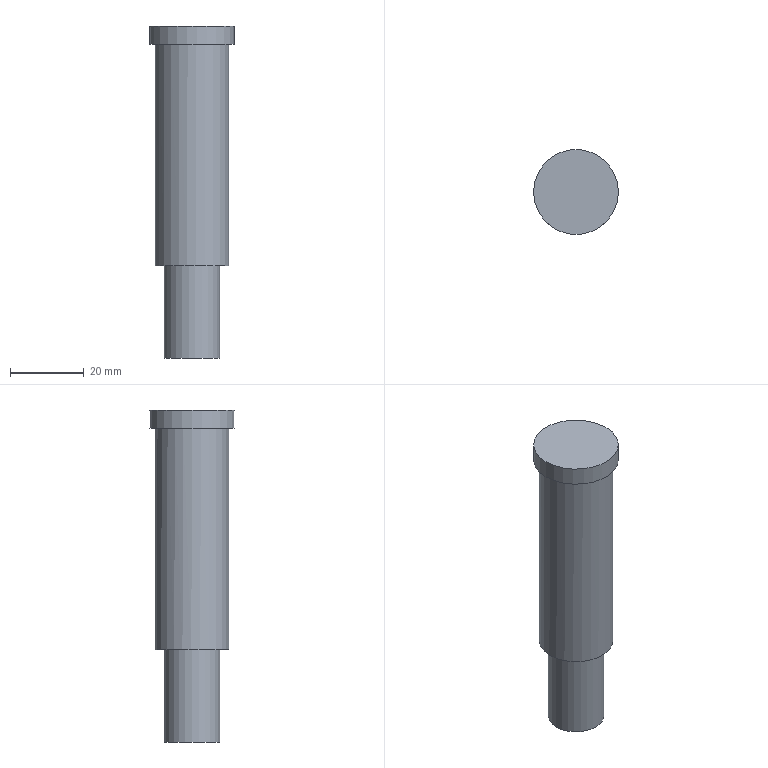Part | NX | features solid 2 | 1 solid | 7 faces | box 23 x 23 x 90 mm | volume 25404 mm3 | plane 4 | cylinder 3 | commonest cylinder face diameters 15.1 x1 20 x1 23 x1
STEP:
#1=CARTESIAN_POINT('',(-704.653,-121.65,86.));
#2=VERTEX_POINT('',#1);
#3=CARTESIAN_POINT('',(-694.993,-124.238,86.));
#4=DIRECTION('',(0.,0.,1.));
#5=DIRECTION('',(-0.9659,0.2588,0.));
#6=AXIS2_PLACEMENT_3D('',#3,#4,#5);
#7=CIRCLE('',#6,10.);
#8=EDGE_CURVE('',#2,#2,#7,.T.);
#9=ORIENTED_EDGE('',*,*,#8,.T.);
#10=EDGE_LOOP('',(#9));
#11=FACE_BOUND('',#10,.T.);
#12=CARTESIAN_POINT('',(-684.993,-124.238,146.));
#13=VERTEX_POINT('',#12);
#14=CARTESIAN_POINT('',(-694.993,-124.238,146.));
#15=DIRECTION('',(0.,0.,1.));
#16=DIRECTION('',(1.,0.,0.));
#17=AXIS2_PLACEMENT_3D('',#14,#15,#16);
#18=CIRCLE('',#17,10.);
#19=EDGE_CURVE('',#13,#13,#18,.T.);
#20=ORIENTED_EDGE('',*,*,#19,.F.);
#21=EDGE_LOOP('',(#20));
#22=FACE_BOUND('',#21,.T.);
#23=CARTESIAN_POINT('',(-694.993,-124.238,141.));
#24=DIRECTION('',(0.,0.,-1.));
#25=DIRECTION('',(0.9659,-0.2588,0.));
#26=AXIS2_PLACEMENT_3D('',#23,#24,#25);
#27=CYLINDRICAL_SURFACE('',#26,10.);
#28=ADVANCED_FACE('',(#11,#22),#27,.T.);
#29=CARTESIAN_POINT('',(-687.443,-124.238,86.));
#30=VERTEX_POINT('',#29);
#31=CARTESIAN_POINT('',(-694.993,-124.238,86.));
#32=DIRECTION('',(0.,0.,1.));
#33=DIRECTION('',(1.,0.,0.));
#34=AXIS2_PLACEMENT_3D('',#31,#32,#33);
#35=CIRCLE('',#34,7.55);
#36=EDGE_CURVE('',#30,#30,#35,.T.);
#37=ORIENTED_EDGE('',*,*,#36,.T.);
#38=EDGE_LOOP('',(#37));
#39=FACE_BOUND('',#38,.T.);
#40=ORIENTED_EDGE('',*,*,#8,.F.);
#41=EDGE_LOOP('',(#40));
#42=FACE_BOUND('',#41,.T.);
#43=CARTESIAN_POINT('',(-694.993,-124.238,86.));
#44=DIRECTION('',(0.,0.,1.));
#45=DIRECTION('',(-0.9659,0.2588,0.));
#46=AXIS2_PLACEMENT_3D('',#43,#44,#45);
#47=PLANE('',#46);
#48=ADVANCED_FACE('',(#39,#42),#47,.F.);
#49=CARTESIAN_POINT('',(-683.493,-124.238,146.));
#50=VERTEX_POINT('',#49);
#51=CARTESIAN_POINT('',(-694.993,-124.238,146.));
#52=DIRECTION('',(0.,0.,1.));
#53=DIRECTION('',(1.,0.,0.));
#54=AXIS2_PLACEMENT_3D('',#51,#52,#53);
#55=CIRCLE('',#54,11.5);
#56=EDGE_CURVE('',#50,#50,#55,.T.);
#57=ORIENTED_EDGE('',*,*,#56,.F.);
#58=EDGE_LOOP('',(#57));
#59=FACE_BOUND('',#58,.T.);
#60=ORIENTED_EDGE('',*,*,#19,.T.);
#61=EDGE_LOOP('',(#60));
#62=FACE_BOUND('',#61,.T.);
#63=CARTESIAN_POINT('',(-694.993,-124.238,146.));
#64=DIRECTION('',(0.,0.,1.));
#65=DIRECTION('',(-0.9659,0.2588,0.));
#66=AXIS2_PLACEMENT_3D('',#63,#64,#65);
#67=PLANE('',#66);
#68=ADVANCED_FACE('',(#59,#62),#67,.F.);
#69=ORIENTED_EDGE('',*,*,#56,.T.);
#70=EDGE_LOOP('',(#69));
#71=FACE_BOUND('',#70,.T.);
#72=CARTESIAN_POINT('',(-683.493,-124.238,151.));
#73=VERTEX_POINT('',#72);
#74=CARTESIAN_POINT('',(-694.993,-124.238,151.));
#75=DIRECTION('',(0.,0.,1.));
#76=DIRECTION('',(1.,0.,0.));
#77=AXIS2_PLACEMENT_3D('',#74,#75,#76);
#78=CIRCLE('',#77,11.5);
#79=EDGE_CURVE('',#73,#73,#78,.T.);
#80=ORIENTED_EDGE('',*,*,#79,.F.);
#81=EDGE_LOOP('',(#80));
#82=FACE_BOUND('',#81,.T.);
#83=CARTESIAN_POINT('',(-694.993,-124.238,136.));
#84=DIRECTION('',(0.,0.,1.));
#85=DIRECTION('',(-0.9659,0.2588,0.));
#86=AXIS2_PLACEMENT_3D('',#83,#84,#85);
#87=CYLINDRICAL_SURFACE('',#86,11.5);
#88=ADVANCED_FACE('',(#71,#82),#87,.T.);
#89=ORIENTED_EDGE('',*,*,#79,.T.);
#90=EDGE_LOOP('',(#89));
#91=FACE_BOUND('',#90,.T.);
#92=CARTESIAN_POINT('',(-694.993,-124.238,151.));
#93=DIRECTION('',(0.,0.,1.));
#94=DIRECTION('',(-0.9659,0.2588,0.));
#95=AXIS2_PLACEMENT_3D('',#92,#93,#94);
#96=PLANE('',#95);
#97=ADVANCED_FACE('',(#91),#96,.T.);
#98=CARTESIAN_POINT('',(-687.443,-124.238,61.));
#99=VERTEX_POINT('',#98);
#100=CARTESIAN_POINT('',(-694.993,-124.238,61.));
#101=DIRECTION('',(0.,0.,1.));
#102=DIRECTION('',(1.,0.,0.));
#103=AXIS2_PLACEMENT_3D('',#100,#101,#102);
#104=CIRCLE('',#103,7.55);
#105=EDGE_CURVE('',#99,#99,#104,.T.);
#106=ORIENTED_EDGE('',*,*,#105,.T.);
#107=EDGE_LOOP('',(#106));
#108=FACE_BOUND('',#107,.T.);
#109=ORIENTED_EDGE('',*,*,#36,.F.);
#110=EDGE_LOOP('',(#109));
#111=FACE_BOUND('',#110,.T.);
#112=CARTESIAN_POINT('',(-694.993,-124.238,61.));
#113=DIRECTION('',(0.,0.,1.));
#114=DIRECTION('',(-0.9659,0.2588,0.));
#115=AXIS2_PLACEMENT_3D('',#112,#113,#114);
#116=CYLINDRICAL_SURFACE('',#115,7.55);
#117=ADVANCED_FACE('',(#108,#111),#116,.T.);
#118=ORIENTED_EDGE('',*,*,#105,.F.);
#119=EDGE_LOOP('',(#118));
#120=FACE_BOUND('',#119,.T.);
#121=CARTESIAN_POINT('',(-694.993,-124.238,61.));
#122=DIRECTION('',(0.,0.,1.));
#123=DIRECTION('',(-0.9659,0.2588,0.));
#124=AXIS2_PLACEMENT_3D('',#121,#122,#123);
#125=PLANE('',#124);
#126=ADVANCED_FACE('',(#120),#125,.F.);
#127=CLOSED_SHELL('',(#28,#48,#68,#88,#97,#117,#126));
#128=MANIFOLD_SOLID_BREP('',#127);
#129=(LENGTH_UNIT()NAMED_UNIT(*)SI_UNIT(.MILLI.,.METRE.));
#130=UNCERTAINTY_MEASURE_WITH_UNIT(LENGTH_MEASURE(0.00001),#129,'','');
#131=(NAMED_UNIT(*)PLANE_ANGLE_UNIT()SI_UNIT($,.RADIAN.));
#132=(NAMED_UNIT(*)SI_UNIT($,.STERADIAN.)SOLID_ANGLE_UNIT());
#133=(GEOMETRIC_REPRESENTATION_CONTEXT(3)GLOBAL_UNCERTAINTY_ASSIGNED_CONTEXT((#130))GLOBAL_UNIT_ASSIGNED_CONTEXT((#129,#131,#132))REPRESENTATION_CONTEXT('',''));
#134=ADVANCED_BREP_SHAPE_REPRESENTATION('',(#128),#133);